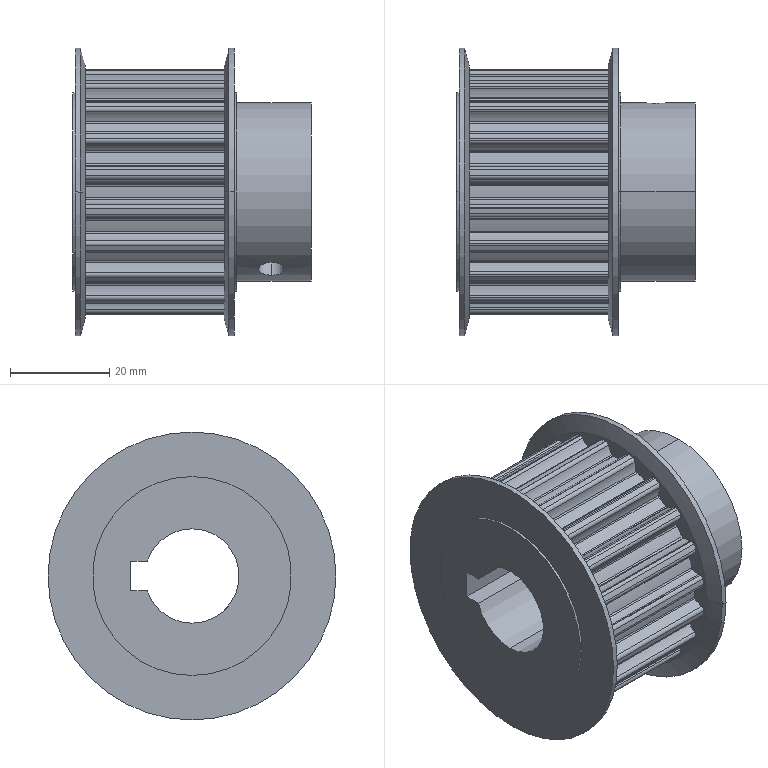Part | SolidWorks | features BaseBody 1 | 1 solid | 212 faces | box 48 x 57.9 x 57.9 mm | volume 58818 mm3 | cylinder 198 | plane 10 | cone 4 | commonest cylinder face diameters 1.5 x50 0.8 x46 10.6 x44 43.9 x21 49.56 x20 5.16 x4